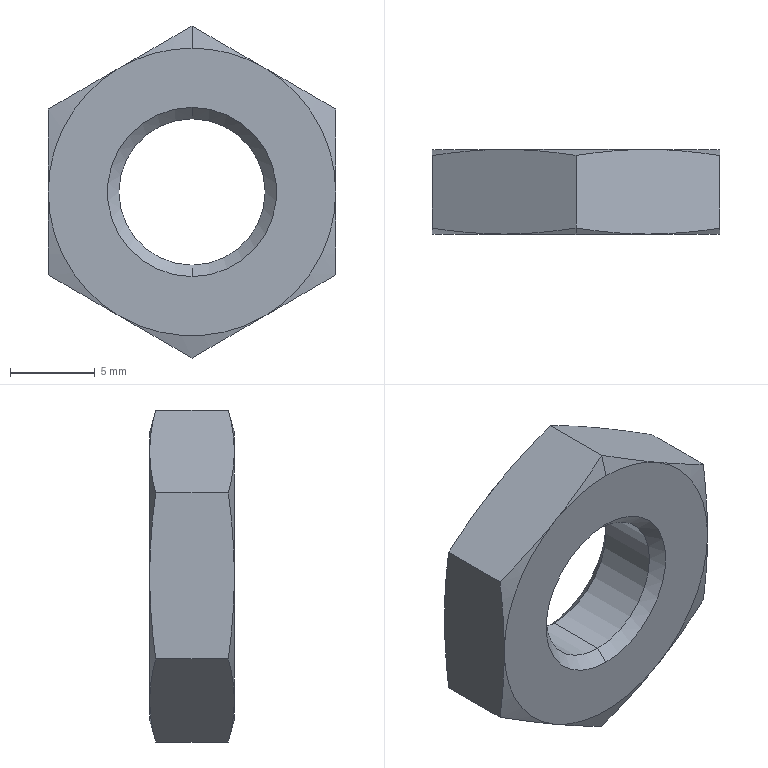Part | STEP file | 1 solid | 28 faces | box 17 x 5 x 19.63 mm | volume 939.625 mm3 | cone 18 | plane 8 | cylinder 2 | commonest cylinder face diameters 8.647 x2